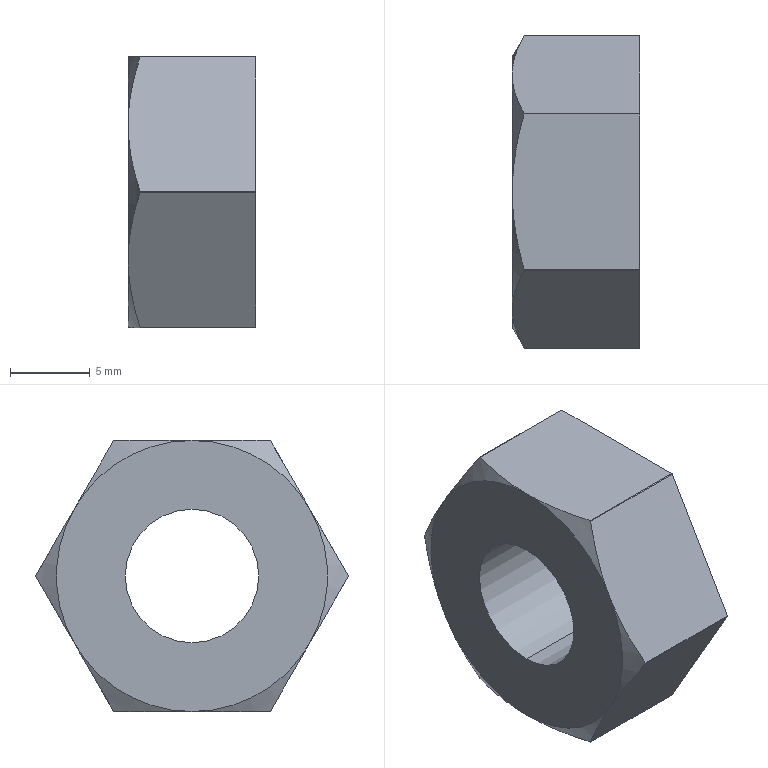Part | SolidWorks | features BaseBody 1 | 1 solid | 24 faces | box 8 x 19.6 x 17 mm | volume 1547 mm3 | cone 8 | cylinder 8 | plane 8 | commonest cylinder face diameters 19.6 x6 8.376 x2
STEP:
#1=CARTESIAN_POINT('',(-0.812,0.,-4.188));
#2=VERTEX_POINT('',#1);
#3=CARTESIAN_POINT('',(-0.812,0.,4.188));
#4=VERTEX_POINT('',#3);
#5=CARTESIAN_POINT('',(-0.812,0.,0.));
#6=DIRECTION('',(-1.,0.,0.));
#7=DIRECTION('',(0.,0.,1.));
#8=AXIS2_PLACEMENT_3D('',#5,#6,#7);
#9=CIRCLE('',#8,4.188);
#10=EDGE_CURVE('',#2,#4,#9,.T.);
#11=ORIENTED_EDGE('',*,*,#10,.T.);
#12=CARTESIAN_POINT('',(0.,0.,5.));
#13=VERTEX_POINT('',#12);
#14=CARTESIAN_POINT('',(0.,0.,5.));
#15=DIRECTION('',(0.7071,0.,0.7071));
#16=VECTOR('',#15,1000.);
#17=LINE('',#14,#16);
#18=EDGE_CURVE('',#4,#13,#17,.T.);
#19=ORIENTED_EDGE('',*,*,#18,.T.);
#20=CARTESIAN_POINT('',(0.,0.,-5.));
#21=VERTEX_POINT('',#20);
#22=CARTESIAN_POINT('',(0.,0.,0.));
#23=DIRECTION('',(-1.,0.,0.));
#24=DIRECTION('',(0.,0.,1.));
#25=AXIS2_PLACEMENT_3D('',#22,#23,#24);
#26=CIRCLE('',#25,5.);
#27=EDGE_CURVE('',#21,#13,#26,.T.);
#28=ORIENTED_EDGE('',*,*,#27,.F.);
#29=CARTESIAN_POINT('',(0.,0.,-5.));
#30=DIRECTION('',(0.7071,0.,-0.7071));
#31=VECTOR('',#30,1000.);
#32=LINE('',#29,#31);
#33=EDGE_CURVE('',#2,#21,#32,.T.);
#34=ORIENTED_EDGE('',*,*,#33,.F.);
#35=EDGE_LOOP('',(#11,#19,#28,#34));
#36=FACE_OUTER_BOUND('',#35,.T.);
#37=CARTESIAN_POINT('',(0.,0.,0.));
#38=DIRECTION('',(1.,0.,0.));
#39=DIRECTION('',(0.,0.,-1.));
#40=AXIS2_PLACEMENT_3D('',#37,#38,#39);
#41=CONICAL_SURFACE('',#40,5.,0.7854);
#42=ADVANCED_FACE('',(#36),#41,.F.);
#43=ORIENTED_EDGE('',*,*,#10,.F.);
#44=CARTESIAN_POINT('',(-8.,0.,-4.188));
#45=VERTEX_POINT('',#44);
#46=CARTESIAN_POINT('',(0.,0.,-4.188));
#47=DIRECTION('',(-1.,0.,0.));
#48=VECTOR('',#47,1000.);
#49=LINE('',#46,#48);
#50=EDGE_CURVE('',#2,#45,#49,.T.);
#51=ORIENTED_EDGE('',*,*,#50,.T.);
#52=CARTESIAN_POINT('',(-8.,0.,4.188));
#53=VERTEX_POINT('',#52);
#54=CARTESIAN_POINT('',(-8.,0.,0.));
#55=DIRECTION('',(-1.,0.,0.));
#56=DIRECTION('',(0.,0.,1.));
#57=AXIS2_PLACEMENT_3D('',#54,#55,#56);
#58=CIRCLE('',#57,4.188);
#59=EDGE_CURVE('',#45,#53,#58,.T.);
#60=ORIENTED_EDGE('',*,*,#59,.T.);
#61=CARTESIAN_POINT('',(0.,0.,4.188));
#62=DIRECTION('',(-1.,0.,0.));
#63=VECTOR('',#62,1000.);
#64=LINE('',#61,#63);
#65=EDGE_CURVE('',#4,#53,#64,.T.);
#66=ORIENTED_EDGE('',*,*,#65,.F.);
#67=EDGE_LOOP('',(#43,#51,#60,#66));
#68=FACE_OUTER_BOUND('',#67,.T.);
#69=CARTESIAN_POINT('',(0.,0.,0.));
#70=DIRECTION('',(-1.,0.,0.));
#71=DIRECTION('',(0.,0.,1.));
#72=AXIS2_PLACEMENT_3D('',#69,#70,#71);
#73=CYLINDRICAL_SURFACE('',#72,4.188);
#74=ADVANCED_FACE('',(#68),#73,.F.);
#75=ORIENTED_EDGE('',*,*,#27,.T.);
#76=CARTESIAN_POINT('',(0.,0.,0.));
#77=DIRECTION('',(-1.,0.,0.));
#78=DIRECTION('',(0.,0.,1.));
#79=AXIS2_PLACEMENT_3D('',#76,#77,#78);
#80=CIRCLE('',#79,5.);
#81=EDGE_CURVE('',#13,#21,#80,.T.);
#82=ORIENTED_EDGE('',*,*,#81,.T.);
#83=EDGE_LOOP('',(#75,#82));
#84=FACE_BOUND('',#83,.T.);
#85=CARTESIAN_POINT('',(0.,9.8,0.02596));
#86=VERTEX_POINT('',#85);
#87=CARTESIAN_POINT('',(0.,4.922,8.474));
#88=VERTEX_POINT('',#87);
#89=CARTESIAN_POINT('',(0.,9.815,0.));
#90=DIRECTION('',(0.,-0.5,0.866));
#91=VECTOR('',#90,1000.);
#92=LINE('',#89,#91);
#93=EDGE_CURVE('',#86,#88,#92,.T.);
#94=ORIENTED_EDGE('',*,*,#93,.T.);
#95=CARTESIAN_POINT('',(0.,4.877,8.5));
#96=VERTEX_POINT('',#95);
#97=CARTESIAN_POINT('',(0.,0.,0.));
#98=DIRECTION('',(-1.,0.,0.));
#99=DIRECTION('',(0.,0.,1.));
#100=AXIS2_PLACEMENT_3D('',#97,#98,#99);
#101=CIRCLE('',#100,9.8);
#102=EDGE_CURVE('',#96,#88,#101,.T.);
#103=ORIENTED_EDGE('',*,*,#102,.F.);
#104=CARTESIAN_POINT('',(0.,-4.877,8.5));
#105=VERTEX_POINT('',#104);
#106=CARTESIAN_POINT('',(0.,4.907,8.5));
#107=DIRECTION('',(0.,-1.,0.));
#108=VECTOR('',#107,1000.);
#109=LINE('',#106,#108);
#110=EDGE_CURVE('',#96,#105,#109,.T.);
#111=ORIENTED_EDGE('',*,*,#110,.T.);
#112=CARTESIAN_POINT('',(0.,-4.922,8.474));
#113=VERTEX_POINT('',#112);
#114=CARTESIAN_POINT('',(0.,0.,0.));
#115=DIRECTION('',(-1.,0.,0.));
#116=DIRECTION('',(0.,0.,1.));
#117=AXIS2_PLACEMENT_3D('',#114,#115,#116);
#118=CIRCLE('',#117,9.8);
#119=EDGE_CURVE('',#113,#105,#118,.T.);
#120=ORIENTED_EDGE('',*,*,#119,.F.);
#121=CARTESIAN_POINT('',(0.,-9.8,0.02596));
#122=VERTEX_POINT('',#121);
#123=CARTESIAN_POINT('',(0.,-4.907,8.5));
#124=DIRECTION('',(0.,-0.5,-0.866));
#125=VECTOR('',#124,1000.);
#126=LINE('',#123,#125);
#127=EDGE_CURVE('',#113,#122,#126,.T.);
#128=ORIENTED_EDGE('',*,*,#127,.T.);
#129=CARTESIAN_POINT('',(0.,-9.8,-0.02596));
#130=VERTEX_POINT('',#129);
#131=CARTESIAN_POINT('',(0.,0.,0.));
#132=DIRECTION('',(-1.,0.,0.));
#133=DIRECTION('',(0.,0.,1.));
#134=AXIS2_PLACEMENT_3D('',#131,#132,#133);
#135=CIRCLE('',#134,9.8);
#136=EDGE_CURVE('',#130,#122,#135,.T.);
#137=ORIENTED_EDGE('',*,*,#136,.F.);
#138=CARTESIAN_POINT('',(0.,-4.922,-8.474));
#139=VERTEX_POINT('',#138);
#140=CARTESIAN_POINT('',(0.,-9.815,0.));
#141=DIRECTION('',(0.,0.5,-0.866));
#142=VECTOR('',#141,1000.);
#143=LINE('',#140,#142);
#144=EDGE_CURVE('',#130,#139,#143,.T.);
#145=ORIENTED_EDGE('',*,*,#144,.T.);
#146=CARTESIAN_POINT('',(0.,-4.877,-8.5));
#147=VERTEX_POINT('',#146);
#148=CARTESIAN_POINT('',(0.,0.,0.));
#149=DIRECTION('',(-1.,0.,0.));
#150=DIRECTION('',(0.,0.,1.));
#151=AXIS2_PLACEMENT_3D('',#148,#149,#150);
#152=CIRCLE('',#151,9.8);
#153=EDGE_CURVE('',#147,#139,#152,.T.);
#154=ORIENTED_EDGE('',*,*,#153,.F.);
#155=CARTESIAN_POINT('',(0.,4.877,-8.5));
#156=VERTEX_POINT('',#155);
#157=CARTESIAN_POINT('',(0.,-4.907,-8.5));
#158=DIRECTION('',(0.,1.,0.));
#159=VECTOR('',#158,1000.);
#160=LINE('',#157,#159);
#161=EDGE_CURVE('',#147,#156,#160,.T.);
#162=ORIENTED_EDGE('',*,*,#161,.T.);
#163=CARTESIAN_POINT('',(0.,4.922,-8.474));
#164=VERTEX_POINT('',#163);
#165=CARTESIAN_POINT('',(0.,0.,0.));
#166=DIRECTION('',(-1.,0.,0.));
#167=DIRECTION('',(0.,0.,1.));
#168=AXIS2_PLACEMENT_3D('',#165,#166,#167);
#169=CIRCLE('',#168,9.8);
#170=EDGE_CURVE('',#164,#156,#169,.T.);
#171=ORIENTED_EDGE('',*,*,#170,.F.);
#172=CARTESIAN_POINT('',(0.,9.8,-0.02596));
#173=VERTEX_POINT('',#172);
#174=CARTESIAN_POINT('',(0.,4.907,-8.5));
#175=DIRECTION('',(0.,0.5,0.866));
#176=VECTOR('',#175,1000.);
#177=LINE('',#174,#176);
#178=EDGE_CURVE('',#164,#173,#177,.T.);
#179=ORIENTED_EDGE('',*,*,#178,.T.);
#180=CARTESIAN_POINT('',(0.,0.,0.));
#181=DIRECTION('',(-1.,0.,0.));
#182=DIRECTION('',(0.,0.,1.));
#183=AXIS2_PLACEMENT_3D('',#180,#181,#182);
#184=CIRCLE('',#183,9.8);
#185=EDGE_CURVE('',#86,#173,#184,.T.);
#186=ORIENTED_EDGE('',*,*,#185,.F.);
#187=EDGE_LOOP('',(#94,#103,#111,#120,#128,#137,#145,#154,#162,#171,#179,#186));
#188=FACE_OUTER_BOUND('',#187,.T.);
#189=CARTESIAN_POINT('',(0.,9.8,0.));
#190=DIRECTION('',(-1.,0.,0.));
#191=DIRECTION('',(0.,0.,1.));
#192=AXIS2_PLACEMENT_3D('',#189,#190,#191);
#193=PLANE('',#192);
#194=ADVANCED_FACE('',(#84,#188),#193,.F.);
#195=CARTESIAN_POINT('',(-7.249,9.8,0.02596));
#196=VERTEX_POINT('',#195);
#197=CARTESIAN_POINT('',(-8.,7.361,4.25));
#198=VERTEX_POINT('',#197);
#199=CARTESIAN_POINT('',(-7.249,9.8,0.02596));
#200=CARTESIAN_POINT('',(-7.479,9.401,0.7171));
#201=CARTESIAN_POINT('',(-7.668,8.999,1.413));
#202=CARTESIAN_POINT('',(-7.929,8.187,2.82));
#203=CARTESIAN_POINT('',(-8.,7.777,3.531));
#204=CARTESIAN_POINT('',(-8.,7.361,4.25));
#205=B_SPLINE_CURVE_WITH_KNOTS('',3,(#199,#200,#201,#202,#203,#204),.UNSPECIFIED.,.F.,.F.,(4,2,4),(0.000000483,0.002468,0.004935),.UNSPECIFIED.);
#206=EDGE_CURVE('',#196,#198,#205,.T.);
#207=ORIENTED_EDGE('',*,*,#206,.F.);
#208=CARTESIAN_POINT('',(-7.249,9.8,-0.02596));
#209=VERTEX_POINT('',#208);
#210=CARTESIAN_POINT('',(-7.249,0.,0.));
#211=DIRECTION('',(-1.,0.,0.));
#212=DIRECTION('',(0.,0.,1.));
#213=AXIS2_PLACEMENT_3D('',#210,#211,#212);
#214=CIRCLE('',#213,9.8);
#215=EDGE_CURVE('',#196,#209,#214,.T.);
#216=ORIENTED_EDGE('',*,*,#215,.T.);
#217=CARTESIAN_POINT('',(-8.,7.361,-4.25));
#218=VERTEX_POINT('',#217);
#219=CARTESIAN_POINT('',(-8.,7.361,-4.25));
#220=CARTESIAN_POINT('',(-8.,7.568,-3.892));
#221=CARTESIAN_POINT('',(-7.982,7.776,-3.532));
#222=CARTESIAN_POINT('',(-7.914,8.187,-2.819));
#223=CARTESIAN_POINT('',(-7.863,8.391,-2.466));
#224=CARTESIAN_POINT('',(-7.667,9.001,-1.41));
#225=CARTESIAN_POINT('',(-7.478,9.402,-0.7153));
#226=CARTESIAN_POINT('',(-7.249,9.8,-0.02596));
#227=B_SPLINE_CURVE_WITH_KNOTS('',3,(#219,#220,#221,#222,#223,#224,#225,#226),.UNSPECIFIED.,.F.,.F.,(4,2,2,4),(0.004935,0.006164,0.007393,0.00985),.UNSPECIFIED.);
#228=EDGE_CURVE('',#218,#209,#227,.T.);
#229=ORIENTED_EDGE('',*,*,#228,.F.);
#230=CARTESIAN_POINT('',(-8.,0.,0.));
#231=DIRECTION('',(-1.,0.,0.));
#232=DIRECTION('',(0.,0.,1.));
#233=AXIS2_PLACEMENT_3D('',#230,#231,#232);
#234=CIRCLE('',#233,8.5);
#235=EDGE_CURVE('',#198,#218,#234,.T.);
#236=ORIENTED_EDGE('',*,*,#235,.F.);
#237=EDGE_LOOP('',(#207,#216,#229,#236));
#238=FACE_OUTER_BOUND('',#237,.T.);
#239=CARTESIAN_POINT('',(-7.249,0.,0.));
#240=DIRECTION('',(1.,0.,0.));
#241=DIRECTION('',(0.,0.,-1.));
#242=AXIS2_PLACEMENT_3D('',#239,#240,#241);
#243=CONICAL_SURFACE('',#242,9.8,1.047);
#244=ADVANCED_FACE('',(#238),#243,.T.);
#245=CARTESIAN_POINT('',(-7.249,4.922,8.474));
#246=VERTEX_POINT('',#245);
#247=CARTESIAN_POINT('',(-8.,7.361,4.25));
#248=CARTESIAN_POINT('',(-8.,7.154,4.608));
#249=CARTESIAN_POINT('',(-7.982,6.946,4.968));
#250=CARTESIAN_POINT('',(-7.914,6.535,5.681));
#251=CARTESIAN_POINT('',(-7.863,6.331,6.034));
#252=CARTESIAN_POINT('',(-7.667,5.722,7.09));
#253=CARTESIAN_POINT('',(-7.478,5.32,7.785));
#254=CARTESIAN_POINT('',(-7.249,4.922,8.474));
#255=B_SPLINE_CURVE_WITH_KNOTS('',3,(#247,#248,#249,#250,#251,#252,#253,#254),.UNSPECIFIED.,.F.,.F.,(4,2,2,4),(0.004935,0.006164,0.007393,0.00985),.UNSPECIFIED.);
#256=EDGE_CURVE('',#198,#246,#255,.T.);
#257=ORIENTED_EDGE('',*,*,#256,.F.);
#258=CARTESIAN_POINT('',(-8.,0.,8.5));
#259=VERTEX_POINT('',#258);
#260=CARTESIAN_POINT('',(-8.,0.,0.));
#261=DIRECTION('',(-1.,0.,0.));
#262=DIRECTION('',(0.,0.,1.));
#263=AXIS2_PLACEMENT_3D('',#260,#261,#262);
#264=CIRCLE('',#263,8.5);
#265=EDGE_CURVE('',#259,#198,#264,.T.);
#266=ORIENTED_EDGE('',*,*,#265,.F.);
#267=CARTESIAN_POINT('',(-7.249,4.877,8.5));
#268=VERTEX_POINT('',#267);
#269=CARTESIAN_POINT('',(-7.249,4.877,8.5));
#270=CARTESIAN_POINT('',(-7.476,4.089,8.5));
#271=CARTESIAN_POINT('',(-7.665,3.29,8.5));
#272=CARTESIAN_POINT('',(-7.928,1.66,8.5));
#273=CARTESIAN_POINT('',(-8.,0.8245,8.5));
#274=CARTESIAN_POINT('',(-8.,0.,8.5));
#275=B_SPLINE_CURVE_WITH_KNOTS('',3,(#269,#270,#271,#272,#273,#274),.UNSPECIFIED.,.F.,.F.,(4,2,4),(0.00363,0.006092,0.008554),.UNSPECIFIED.);
#276=EDGE_CURVE('',#268,#259,#275,.T.);
#277=ORIENTED_EDGE('',*,*,#276,.F.);
#278=CARTESIAN_POINT('',(-7.249,0.,0.));
#279=DIRECTION('',(-1.,0.,0.));
#280=DIRECTION('',(0.,0.,1.));
#281=AXIS2_PLACEMENT_3D('',#278,#279,#280);
#282=CIRCLE('',#281,9.8);
#283=EDGE_CURVE('',#268,#246,#282,.T.);
#284=ORIENTED_EDGE('',*,*,#283,.T.);
#285=EDGE_LOOP('',(#257,#266,#277,#284));
#286=FACE_OUTER_BOUND('',#285,.T.);
#287=CARTESIAN_POINT('',(-7.249,0.,0.));
#288=DIRECTION('',(1.,0.,0.));
#289=DIRECTION('',(0.,0.,-1.));
#290=AXIS2_PLACEMENT_3D('',#287,#288,#289);
#291=CONICAL_SURFACE('',#290,9.8,1.047);
#292=ADVANCED_FACE('',(#286),#291,.T.);
#293=CARTESIAN_POINT('',(-7.249,4.922,-8.474));
#294=VERTEX_POINT('',#293);
#295=CARTESIAN_POINT('',(-7.249,4.922,-8.474));
#296=CARTESIAN_POINT('',(-7.479,5.322,-7.783));
#297=CARTESIAN_POINT('',(-7.668,5.723,-7.087));
#298=CARTESIAN_POINT('',(-7.929,6.536,-5.68));
#299=CARTESIAN_POINT('',(-8.,6.946,-4.969));
#300=CARTESIAN_POINT('',(-8.,7.361,-4.25));
#301=B_SPLINE_CURVE_WITH_KNOTS('',3,(#295,#296,#297,#298,#299,#300),.UNSPECIFIED.,.F.,.F.,(4,2,4),(0.000000717,0.002468,0.004935),.UNSPECIFIED.);
#302=EDGE_CURVE('',#294,#218,#301,.T.);
#303=ORIENTED_EDGE('',*,*,#302,.F.);
#304=CARTESIAN_POINT('',(-7.249,4.877,-8.5));
#305=VERTEX_POINT('',#304);
#306=CARTESIAN_POINT('',(-7.249,0.,0.));
#307=DIRECTION('',(-1.,0.,0.));
#308=DIRECTION('',(0.,0.,1.));
#309=AXIS2_PLACEMENT_3D('',#306,#307,#308);
#310=CIRCLE('',#309,9.8);
#311=EDGE_CURVE('',#294,#305,#310,.T.);
#312=ORIENTED_EDGE('',*,*,#311,.T.);
#313=CARTESIAN_POINT('',(-8.,0.,-8.5));
#314=VERTEX_POINT('',#313);
#315=CARTESIAN_POINT('',(-8.,0.,-8.5));
#316=CARTESIAN_POINT('',(-8.,0.8245,-8.5));
#317=CARTESIAN_POINT('',(-7.928,1.66,-8.5));
#318=CARTESIAN_POINT('',(-7.665,3.29,-8.5));
#319=CARTESIAN_POINT('',(-7.476,4.089,-8.5));
#320=CARTESIAN_POINT('',(-7.249,4.877,-8.5));
#321=B_SPLINE_CURVE_WITH_KNOTS('',3,(#315,#316,#317,#318,#319,#320),.UNSPECIFIED.,.F.,.F.,(4,2,4),(0.01372,0.01619,0.01866),.UNSPECIFIED.);
#322=EDGE_CURVE('',#314,#305,#321,.T.);
#323=ORIENTED_EDGE('',*,*,#322,.F.);
#324=CARTESIAN_POINT('',(-8.,0.,0.));
#325=DIRECTION('',(-1.,0.,0.));
#326=DIRECTION('',(0.,0.,1.));
#327=AXIS2_PLACEMENT_3D('',#324,#325,#326);
#328=CIRCLE('',#327,8.5);
#329=EDGE_CURVE('',#218,#314,#328,.T.);
#330=ORIENTED_EDGE('',*,*,#329,.F.);
#331=EDGE_LOOP('',(#303,#312,#323,#330));
#332=FACE_OUTER_BOUND('',#331,.T.);
#333=CARTESIAN_POINT('',(-7.249,0.,0.));
#334=DIRECTION('',(1.,0.,0.));
#335=DIRECTION('',(0.,0.,-1.));
#336=AXIS2_PLACEMENT_3D('',#333,#334,#335);
#337=CONICAL_SURFACE('',#336,9.8,1.047);
#338=ADVANCED_FACE('',(#332),#337,.T.);
#339=CARTESIAN_POINT('',(-7.249,-4.877,-8.5));
#340=VERTEX_POINT('',#339);
#341=CARTESIAN_POINT('',(-7.249,-4.877,-8.5));
#342=CARTESIAN_POINT('',(-7.477,-4.084,-8.5));
#343=CARTESIAN_POINT('',(-7.669,-3.271,-8.5));
#344=CARTESIAN_POINT('',(-7.93,-1.643,-8.5));
#345=CARTESIAN_POINT('',(-8.,-0.8241,-8.5));
#346=CARTESIAN_POINT('',(-8.,0.,-8.5));
#347=B_SPLINE_CURVE_WITH_KNOTS('',3,(#341,#342,#343,#344,#345,#346),.UNSPECIFIED.,.F.,.F.,(4,2,4),(0.008785,0.01125,0.01372),.UNSPECIFIED.);
#348=EDGE_CURVE('',#340,#314,#347,.T.);
#349=ORIENTED_EDGE('',*,*,#348,.F.);
#350=CARTESIAN_POINT('',(-7.249,-4.922,-8.474));
#351=VERTEX_POINT('',#350);
#352=CARTESIAN_POINT('',(-7.249,0.,0.));
#353=DIRECTION('',(-1.,0.,0.));
#354=DIRECTION('',(0.,0.,1.));
#355=AXIS2_PLACEMENT_3D('',#352,#353,#354);
#356=CIRCLE('',#355,9.8);
#357=EDGE_CURVE('',#340,#351,#356,.T.);
#358=ORIENTED_EDGE('',*,*,#357,.T.);
#359=CARTESIAN_POINT('',(-8.,-7.361,-4.25));
#360=VERTEX_POINT('',#359);
#361=CARTESIAN_POINT('',(-8.,-7.361,-4.25));
#362=CARTESIAN_POINT('',(-8.,-7.154,-4.608));
#363=CARTESIAN_POINT('',(-7.982,-6.946,-4.968));
#364=CARTESIAN_POINT('',(-7.914,-6.535,-5.681));
#365=CARTESIAN_POINT('',(-7.863,-6.331,-6.034));
#366=CARTESIAN_POINT('',(-7.667,-5.722,-7.09));
#367=CARTESIAN_POINT('',(-7.478,-5.32,-7.785));
#368=CARTESIAN_POINT('',(-7.249,-4.922,-8.474));
#369=B_SPLINE_CURVE_WITH_KNOTS('',3,(#361,#362,#363,#364,#365,#366,#367,#368),.UNSPECIFIED.,.F.,.F.,(4,2,2,4),(0.004935,0.006164,0.007393,0.00985),.UNSPECIFIED.);
#370=EDGE_CURVE('',#360,#351,#369,.T.);
#371=ORIENTED_EDGE('',*,*,#370,.F.);
#372=CARTESIAN_POINT('',(-8.,0.,0.));
#373=DIRECTION('',(-1.,0.,0.));
#374=DIRECTION('',(0.,0.,1.));
#375=AXIS2_PLACEMENT_3D('',#372,#373,#374);
#376=CIRCLE('',#375,8.5);
#377=EDGE_CURVE('',#314,#360,#376,.T.);
#378=ORIENTED_EDGE('',*,*,#377,.F.);
#379=EDGE_LOOP('',(#349,#358,#371,#378));
#380=FACE_OUTER_BOUND('',#379,.T.);
#381=CARTESIAN_POINT('',(-7.249,0.,0.));
#382=DIRECTION('',(1.,0.,0.));
#383=DIRECTION('',(0.,0.,-1.));
#384=AXIS2_PLACEMENT_3D('',#381,#382,#383);
#385=CONICAL_SURFACE('',#384,9.8,1.047);
#386=ADVANCED_FACE('',(#380),#385,.T.);
#387=CARTESIAN_POINT('',(-7.249,-9.8,-0.02596));
#388=VERTEX_POINT('',#387);
#389=CARTESIAN_POINT('',(-7.249,-9.8,-0.02596));
#390=CARTESIAN_POINT('',(-7.479,-9.401,-0.7171));
#391=CARTESIAN_POINT('',(-7.668,-8.999,-1.413));
#392=CARTESIAN_POINT('',(-7.929,-8.187,-2.82));
#393=CARTESIAN_POINT('',(-8.,-7.777,-3.531));
#394=CARTESIAN_POINT('',(-8.,-7.361,-4.25));
#395=B_SPLINE_CURVE_WITH_KNOTS('',3,(#389,#390,#391,#392,#393,#394),.UNSPECIFIED.,.F.,.F.,(4,2,4),(0.000000483,0.002468,0.004935),.UNSPECIFIED.);
#396=EDGE_CURVE('',#388,#360,#395,.T.);
#397=ORIENTED_EDGE('',*,*,#396,.F.);
#398=CARTESIAN_POINT('',(-7.249,-9.8,0.02596));
#399=VERTEX_POINT('',#398);
#400=CARTESIAN_POINT('',(-7.249,0.,0.));
#401=DIRECTION('',(-1.,0.,0.));
#402=DIRECTION('',(0.,0.,1.));
#403=AXIS2_PLACEMENT_3D('',#400,#401,#402);
#404=CIRCLE('',#403,9.8);
#405=EDGE_CURVE('',#388,#399,#404,.T.);
#406=ORIENTED_EDGE('',*,*,#405,.T.);
#407=CARTESIAN_POINT('',(-8.,-7.361,4.25));
#408=VERTEX_POINT('',#407);
#409=CARTESIAN_POINT('',(-8.,-7.361,4.25));
#410=CARTESIAN_POINT('',(-8.,-7.568,3.892));
#411=CARTESIAN_POINT('',(-7.982,-7.776,3.532));
#412=CARTESIAN_POINT('',(-7.914,-8.187,2.819));
#413=CARTESIAN_POINT('',(-7.863,-8.391,2.466));
#414=CARTESIAN_POINT('',(-7.667,-9.001,1.41));
#415=CARTESIAN_POINT('',(-7.478,-9.402,0.7153));
#416=CARTESIAN_POINT('',(-7.249,-9.8,0.02596));
#417=B_SPLINE_CURVE_WITH_KNOTS('',3,(#409,#410,#411,#412,#413,#414,#415,#416),.UNSPECIFIED.,.F.,.F.,(4,2,2,4),(0.004935,0.006164,0.007393,0.00985),.UNSPECIFIED.);
#418=EDGE_CURVE('',#408,#399,#417,.T.);
#419=ORIENTED_EDGE('',*,*,#418,.F.);
#420=CARTESIAN_POINT('',(-8.,0.,0.));
#421=DIRECTION('',(-1.,0.,0.));
#422=DIRECTION('',(0.,0.,1.));
#423=AXIS2_PLACEMENT_3D('',#420,#421,#422);
#424=CIRCLE('',#423,8.5);
#425=EDGE_CURVE('',#360,#408,#424,.T.);
#426=ORIENTED_EDGE('',*,*,#425,.F.);
#427=EDGE_LOOP('',(#397,#406,#419,#426));
#428=FACE_OUTER_BOUND('',#427,.T.);
#429=CARTESIAN_POINT('',(-7.249,0.,0.));
#430=DIRECTION('',(1.,0.,0.));
#431=DIRECTION('',(0.,0.,-1.));
#432=AXIS2_PLACEMENT_3D('',#429,#430,#431);
#433=CONICAL_SURFACE('',#432,9.8,1.047);
#434=ADVANCED_FACE('',(#428),#433,.T.);
#435=CARTESIAN_POINT('',(-7.249,-4.922,8.474));
#436=VERTEX_POINT('',#435);
#437=CARTESIAN_POINT('',(-7.249,-4.922,8.474));
#438=CARTESIAN_POINT('',(-7.479,-5.322,7.783));
#439=CARTESIAN_POINT('',(-7.668,-5.723,7.087));
#440=CARTESIAN_POINT('',(-7.929,-6.536,5.68));
#441=CARTESIAN_POINT('',(-8.,-6.946,4.969));
#442=CARTESIAN_POINT('',(-8.,-7.361,4.25));
#443=B_SPLINE_CURVE_WITH_KNOTS('',3,(#437,#438,#439,#440,#441,#442),.UNSPECIFIED.,.F.,.F.,(4,2,4),(0.000000717,0.002468,0.004935),.UNSPECIFIED.);
#444=EDGE_CURVE('',#436,#408,#443,.T.);
#445=ORIENTED_EDGE('',*,*,#444,.F.);
#446=CARTESIAN_POINT('',(-7.249,-4.877,8.5));
#447=VERTEX_POINT('',#446);
#448=CARTESIAN_POINT('',(-7.249,0.,0.));
#449=DIRECTION('',(-1.,0.,0.));
#450=DIRECTION('',(0.,0.,1.));
#451=AXIS2_PLACEMENT_3D('',#448,#449,#450);
#452=CIRCLE('',#451,9.8);
#453=EDGE_CURVE('',#436,#447,#452,.T.);
#454=ORIENTED_EDGE('',*,*,#453,.T.);
#455=CARTESIAN_POINT('',(-8.,0.,8.5));
#456=CARTESIAN_POINT('',(-8.,-0.8241,8.5));
#457=CARTESIAN_POINT('',(-7.93,-1.643,8.5));
#458=CARTESIAN_POINT('',(-7.669,-3.271,8.5));
#459=CARTESIAN_POINT('',(-7.477,-4.084,8.5));
#460=CARTESIAN_POINT('',(-7.249,-4.877,8.5));
#461=B_SPLINE_CURVE_WITH_KNOTS('',3,(#455,#456,#457,#458,#459,#460),.UNSPECIFIED.,.F.,.F.,(4,2,4),(0.008554,0.01101,0.01347),.UNSPECIFIED.);
#462=EDGE_CURVE('',#259,#447,#461,.T.);
#463=ORIENTED_EDGE('',*,*,#462,.F.);
#464=CARTESIAN_POINT('',(-8.,0.,0.));
#465=DIRECTION('',(-1.,0.,0.));
#466=DIRECTION('',(0.,0.,1.));
#467=AXIS2_PLACEMENT_3D('',#464,#465,#466);
#468=CIRCLE('',#467,8.5);
#469=EDGE_CURVE('',#408,#259,#468,.T.);
#470=ORIENTED_EDGE('',*,*,#469,.F.);
#471=EDGE_LOOP('',(#445,#454,#463,#470));
#472=FACE_OUTER_BOUND('',#471,.T.);
#473=CARTESIAN_POINT('',(-7.249,0.,0.));
#474=DIRECTION('',(1.,0.,0.));
#475=DIRECTION('',(0.,0.,-1.));
#476=AXIS2_PLACEMENT_3D('',#473,#474,#475);
#477=CONICAL_SURFACE('',#476,9.8,1.047);
#478=ADVANCED_FACE('',(#472),#477,.T.);
#479=CARTESIAN_POINT('',(0.,9.8,0.02596));
#480=DIRECTION('',(-1.,0.,0.));
#481=VECTOR('',#480,1000.);
#482=LINE('',#479,#481);
#483=EDGE_CURVE('',#86,#196,#482,.T.);
#484=ORIENTED_EDGE('',*,*,#483,.F.);
#485=ORIENTED_EDGE('',*,*,#185,.T.);
#486=CARTESIAN_POINT('',(0.,9.8,-0.02596));
#487=DIRECTION('',(1.,0.,0.));
#488=VECTOR('',#487,1000.);
#489=LINE('',#486,#488);
#490=EDGE_CURVE('',#209,#173,#489,.T.);
#491=ORIENTED_EDGE('',*,*,#490,.F.);
#492=ORIENTED_EDGE('',*,*,#215,.F.);
#493=EDGE_LOOP('',(#484,#485,#491,#492));
#494=FACE_OUTER_BOUND('',#493,.T.);
#495=CARTESIAN_POINT('',(0.,0.,0.));
#496=DIRECTION('',(-1.,0.,0.));
#497=DIRECTION('',(0.,0.,1.));
#498=AXIS2_PLACEMENT_3D('',#495,#496,#497);
#499=CYLINDRICAL_SURFACE('',#498,9.8);
#500=ADVANCED_FACE('',(#494),#499,.T.);
#501=CARTESIAN_POINT('',(0.,4.922,8.474));
#502=DIRECTION('',(1.,0.,0.));
#503=VECTOR('',#502,1000.);
#504=LINE('',#501,#503);
#505=EDGE_CURVE('',#246,#88,#504,.T.);
#506=ORIENTED_EDGE('',*,*,#505,.F.);
#507=ORIENTED_EDGE('',*,*,#283,.F.);
#508=CARTESIAN_POINT('',(0.,4.877,8.5));
#509=DIRECTION('',(-1.,0.,0.));
#510=VECTOR('',#509,1000.);
#511=LINE('',#508,#510);
#512=EDGE_CURVE('',#96,#268,#511,.T.);
#513=ORIENTED_EDGE('',*,*,#512,.F.);
#514=ORIENTED_EDGE('',*,*,#102,.T.);
#515=EDGE_LOOP('',(#506,#507,#513,#514));
#516=FACE_OUTER_BOUND('',#515,.T.);
#517=CARTESIAN_POINT('',(0.,0.,0.));
#518=DIRECTION('',(-1.,0.,0.));
#519=DIRECTION('',(0.,0.,1.));
#520=AXIS2_PLACEMENT_3D('',#517,#518,#519);
#521=CYLINDRICAL_SURFACE('',#520,9.8);
#522=ADVANCED_FACE('',(#516),#521,.T.);
#523=CARTESIAN_POINT('',(0.,4.922,-8.474));
#524=DIRECTION('',(-1.,0.,0.));
#525=VECTOR('',#524,1000.);
#526=LINE('',#523,#525);
#527=EDGE_CURVE('',#164,#294,#526,.T.);
#528=ORIENTED_EDGE('',*,*,#527,.F.);
#529=ORIENTED_EDGE('',*,*,#170,.T.);
#530=CARTESIAN_POINT('',(0.,4.877,-8.5));
#531=DIRECTION('',(1.,0.,0.));
#532=VECTOR('',#531,1000.);
#533=LINE('',#530,#532);
#534=EDGE_CURVE('',#305,#156,#533,.T.);
#535=ORIENTED_EDGE('',*,*,#534,.F.);
#536=ORIENTED_EDGE('',*,*,#311,.F.);
#537=EDGE_LOOP('',(#528,#529,#535,#536));
#538=FACE_OUTER_BOUND('',#537,.T.);
#539=CARTESIAN_POINT('',(0.,0.,0.));
#540=DIRECTION('',(-1.,0.,0.));
#541=DIRECTION('',(0.,0.,1.));
#542=AXIS2_PLACEMENT_3D('',#539,#540,#541);
#543=CYLINDRICAL_SURFACE('',#542,9.8);
#544=ADVANCED_FACE('',(#538),#543,.T.);
#545=CARTESIAN_POINT('',(0.,-4.877,-8.5));
#546=DIRECTION('',(-1.,0.,0.));
#547=VECTOR('',#546,1000.);
#548=LINE('',#545,#547);
#549=EDGE_CURVE('',#147,#340,#548,.T.);
#550=ORIENTED_EDGE('',*,*,#549,.F.);
#551=ORIENTED_EDGE('',*,*,#153,.T.);
#552=CARTESIAN_POINT('',(0.,-4.922,-8.474));
#553=DIRECTION('',(1.,0.,0.));
#554=VECTOR('',#553,1000.);
#555=LINE('',#552,#554);
#556=EDGE_CURVE('',#351,#139,#555,.T.);
#557=ORIENTED_EDGE('',*,*,#556,.F.);
#558=ORIENTED_EDGE('',*,*,#357,.F.);
#559=EDGE_LOOP('',(#550,#551,#557,#558));
#560=FACE_OUTER_BOUND('',#559,.T.);
#561=CARTESIAN_POINT('',(0.,0.,0.));
#562=DIRECTION('',(-1.,0.,0.));
#563=DIRECTION('',(0.,0.,1.));
#564=AXIS2_PLACEMENT_3D('',#561,#562,#563);
#565=CYLINDRICAL_SURFACE('',#564,9.8);
#566=ADVANCED_FACE('',(#560),#565,.T.);
#567=CARTESIAN_POINT('',(0.,-9.8,-0.02596));
#568=DIRECTION('',(-1.,0.,0.));
#569=VECTOR('',#568,1000.);
#570=LINE('',#567,#569);
#571=EDGE_CURVE('',#130,#388,#570,.T.);
#572=ORIENTED_EDGE('',*,*,#571,.F.);
#573=ORIENTED_EDGE('',*,*,#136,.T.);
#574=CARTESIAN_POINT('',(0.,-9.8,0.02596));
#575=DIRECTION('',(1.,0.,0.));
#576=VECTOR('',#575,1000.);
#577=LINE('',#574,#576);
#578=EDGE_CURVE('',#399,#122,#577,.T.);
#579=ORIENTED_EDGE('',*,*,#578,.F.);
#580=ORIENTED_EDGE('',*,*,#405,.F.);
#581=EDGE_LOOP('',(#572,#573,#579,#580));
#582=FACE_OUTER_BOUND('',#581,.T.);
#583=CARTESIAN_POINT('',(0.,0.,0.));
#584=DIRECTION('',(-1.,0.,0.));
#585=DIRECTION('',(0.,0.,1.));
#586=AXIS2_PLACEMENT_3D('',#583,#584,#585);
#587=CYLINDRICAL_SURFACE('',#586,9.8);
#588=ADVANCED_FACE('',(#582),#587,.T.);
#589=CARTESIAN_POINT('',(0.,-4.922,8.474));
#590=DIRECTION('',(-1.,0.,0.));
#591=VECTOR('',#590,1000.);
#592=LINE('',#589,#591);
#593=EDGE_CURVE('',#113,#436,#592,.T.);
#594=ORIENTED_EDGE('',*,*,#593,.F.);
#595=ORIENTED_EDGE('',*,*,#119,.T.);
#596=CARTESIAN_POINT('',(0.,-4.877,8.5));
#597=DIRECTION('',(1.,0.,0.));
#598=VECTOR('',#597,1000.);
#599=LINE('',#596,#598);
#600=EDGE_CURVE('',#447,#105,#599,.T.);
#601=ORIENTED_EDGE('',*,*,#600,.F.);
#602=ORIENTED_EDGE('',*,*,#453,.F.);
#603=EDGE_LOOP('',(#594,#595,#601,#602));
#604=FACE_OUTER_BOUND('',#603,.T.);
#605=CARTESIAN_POINT('',(0.,0.,0.));
#606=DIRECTION('',(-1.,0.,0.));
#607=DIRECTION('',(0.,0.,1.));
#608=AXIS2_PLACEMENT_3D('',#605,#606,#607);
#609=CYLINDRICAL_SURFACE('',#608,9.8);
#610=ADVANCED_FACE('',(#604),#609,.T.);
#611=ORIENTED_EDGE('',*,*,#265,.T.);
#612=ORIENTED_EDGE('',*,*,#235,.T.);
#613=ORIENTED_EDGE('',*,*,#329,.T.);
#614=ORIENTED_EDGE('',*,*,#377,.T.);
#615=ORIENTED_EDGE('',*,*,#425,.T.);
#616=ORIENTED_EDGE('',*,*,#469,.T.);
#617=EDGE_LOOP('',(#611,#612,#613,#614,#615,#616));
#618=FACE_OUTER_BOUND('',#617,.T.);
#619=CARTESIAN_POINT('',(-8.,0.,0.));
#620=DIRECTION('',(-1.,0.,0.));
#621=DIRECTION('',(0.,0.,1.));
#622=AXIS2_PLACEMENT_3D('',#619,#620,#621);
#623=CIRCLE('',#622,4.188);
#624=EDGE_CURVE('',#53,#45,#623,.T.);
#625=ORIENTED_EDGE('',*,*,#624,.F.);
#626=ORIENTED_EDGE('',*,*,#59,.F.);
#627=EDGE_LOOP('',(#625,#626));
#628=FACE_BOUND('',#627,.T.);
#629=CARTESIAN_POINT('',(-8.,0.,0.));
#630=DIRECTION('',(1.,0.,0.));
#631=DIRECTION('',(0.,0.,-1.));
#632=AXIS2_PLACEMENT_3D('',#629,#630,#631);
#633=PLANE('',#632);
#634=ADVANCED_FACE('',(#618,#628),#633,.F.);
#635=ORIENTED_EDGE('',*,*,#50,.F.);
#636=CARTESIAN_POINT('',(-0.812,0.,0.));
#637=DIRECTION('',(-1.,0.,0.));
#638=DIRECTION('',(0.,0.,1.));
#639=AXIS2_PLACEMENT_3D('',#636,#637,#638);
#640=CIRCLE('',#639,4.188);
#641=EDGE_CURVE('',#4,#2,#640,.T.);
#642=ORIENTED_EDGE('',*,*,#641,.F.);
#643=ORIENTED_EDGE('',*,*,#65,.T.);
#644=ORIENTED_EDGE('',*,*,#624,.T.);
#645=EDGE_LOOP('',(#635,#642,#643,#644));
#646=FACE_OUTER_BOUND('',#645,.T.);
#647=CARTESIAN_POINT('',(0.,0.,0.));
#648=DIRECTION('',(-1.,0.,0.));
#649=DIRECTION('',(0.,0.,1.));
#650=AXIS2_PLACEMENT_3D('',#647,#648,#649);
#651=CYLINDRICAL_SURFACE('',#650,4.188);
#652=ADVANCED_FACE('',(#646),#651,.F.);
#653=ORIENTED_EDGE('',*,*,#18,.F.);
#654=ORIENTED_EDGE('',*,*,#641,.T.);
#655=ORIENTED_EDGE('',*,*,#33,.T.);
#656=ORIENTED_EDGE('',*,*,#81,.F.);
#657=EDGE_LOOP('',(#653,#654,#655,#656));
#658=FACE_OUTER_BOUND('',#657,.T.);
#659=CARTESIAN_POINT('',(0.,0.,0.));
#660=DIRECTION('',(1.,0.,0.));
#661=DIRECTION('',(0.,0.,-1.));
#662=AXIS2_PLACEMENT_3D('',#659,#660,#661);
#663=CONICAL_SURFACE('',#662,5.,0.7854);
#664=ADVANCED_FACE('',(#658),#663,.F.);
#665=ORIENTED_EDGE('',*,*,#512,.T.);
#666=ORIENTED_EDGE('',*,*,#276,.T.);
#667=ORIENTED_EDGE('',*,*,#462,.T.);
#668=ORIENTED_EDGE('',*,*,#600,.T.);
#669=ORIENTED_EDGE('',*,*,#110,.F.);
#670=EDGE_LOOP('',(#665,#666,#667,#668,#669));
#671=FACE_OUTER_BOUND('',#670,.T.);
#672=CARTESIAN_POINT('',(-8.,4.907,8.5));
#673=DIRECTION('',(0.,0.,1.));
#674=DIRECTION('',(1.,0.,0.));
#675=AXIS2_PLACEMENT_3D('',#672,#673,#674);
#676=PLANE('',#675);
#677=ADVANCED_FACE('',(#671),#676,.T.);
#678=ORIENTED_EDGE('',*,*,#593,.T.);
#679=ORIENTED_EDGE('',*,*,#444,.T.);
#680=ORIENTED_EDGE('',*,*,#418,.T.);
#681=ORIENTED_EDGE('',*,*,#578,.T.);
#682=ORIENTED_EDGE('',*,*,#127,.F.);
#683=EDGE_LOOP('',(#678,#679,#680,#681,#682));
#684=FACE_OUTER_BOUND('',#683,.T.);
#685=CARTESIAN_POINT('',(-8.,-4.907,8.5));
#686=DIRECTION('',(0.,-0.866,0.5));
#687=DIRECTION('',(0.,-0.5,-0.866));
#688=AXIS2_PLACEMENT_3D('',#685,#686,#687);
#689=PLANE('',#688);
#690=ADVANCED_FACE('',(#684),#689,.T.);
#691=ORIENTED_EDGE('',*,*,#571,.T.);
#692=ORIENTED_EDGE('',*,*,#396,.T.);
#693=ORIENTED_EDGE('',*,*,#370,.T.);
#694=ORIENTED_EDGE('',*,*,#556,.T.);
#695=ORIENTED_EDGE('',*,*,#144,.F.);
#696=EDGE_LOOP('',(#691,#692,#693,#694,#695));
#697=FACE_OUTER_BOUND('',#696,.T.);
#698=CARTESIAN_POINT('',(-8.,-9.815,0.));
#699=DIRECTION('',(0.,-0.866,-0.5));
#700=DIRECTION('',(0.,0.5,-0.866));
#701=AXIS2_PLACEMENT_3D('',#698,#699,#700);
#702=PLANE('',#701);
#703=ADVANCED_FACE('',(#697),#702,.T.);
#704=ORIENTED_EDGE('',*,*,#549,.T.);
#705=ORIENTED_EDGE('',*,*,#348,.T.);
#706=ORIENTED_EDGE('',*,*,#322,.T.);
#707=ORIENTED_EDGE('',*,*,#534,.T.);
#708=ORIENTED_EDGE('',*,*,#161,.F.);
#709=EDGE_LOOP('',(#704,#705,#706,#707,#708));
#710=FACE_OUTER_BOUND('',#709,.T.);
#711=CARTESIAN_POINT('',(-8.,-4.907,-8.5));
#712=DIRECTION('',(0.,0.,-1.));
#713=DIRECTION('',(-1.,0.,0.));
#714=AXIS2_PLACEMENT_3D('',#711,#712,#713);
#715=PLANE('',#714);
#716=ADVANCED_FACE('',(#710),#715,.T.);
#717=ORIENTED_EDGE('',*,*,#527,.T.);
#718=ORIENTED_EDGE('',*,*,#302,.T.);
#719=ORIENTED_EDGE('',*,*,#228,.T.);
#720=ORIENTED_EDGE('',*,*,#490,.T.);
#721=ORIENTED_EDGE('',*,*,#178,.F.);
#722=EDGE_LOOP('',(#717,#718,#719,#720,#721));
#723=FACE_OUTER_BOUND('',#722,.T.);
#724=CARTESIAN_POINT('',(-8.,4.907,-8.5));
#725=DIRECTION('',(0.,0.866,-0.5));
#726=DIRECTION('',(0.,0.5,0.866));
#727=AXIS2_PLACEMENT_3D('',#724,#725,#726);
#728=PLANE('',#727);
#729=ADVANCED_FACE('',(#723),#728,.T.);
#730=ORIENTED_EDGE('',*,*,#483,.T.);
#731=ORIENTED_EDGE('',*,*,#206,.T.);
#732=ORIENTED_EDGE('',*,*,#256,.T.);
#733=ORIENTED_EDGE('',*,*,#505,.T.);
#734=ORIENTED_EDGE('',*,*,#93,.F.);
#735=EDGE_LOOP('',(#730,#731,#732,#733,#734));
#736=FACE_OUTER_BOUND('',#735,.T.);
#737=CARTESIAN_POINT('',(-8.,9.815,0.));
#738=DIRECTION('',(0.,0.866,0.5));
#739=DIRECTION('',(0.,-0.5,0.866));
#740=AXIS2_PLACEMENT_3D('',#737,#738,#739);
#741=PLANE('',#740);
#742=ADVANCED_FACE('',(#736),#741,.T.);
#743=CLOSED_SHELL('',(#42,#74,#194,#244,#292,#338,#386,#434,#478,#500,#522,#544,#566,#588,#610,#634,#652,#664,#677,#690,#703,#716,#729,#742));
#744=MANIFOLD_SOLID_BREP('',#743);
#745=CARTESIAN_POINT('',(0.,0.,0.));
#746=DIRECTION('',(0.,0.,1.));
#747=DIRECTION('',(1.,0.,0.));
#748=AXIS2_PLACEMENT_3D('',#745,#746,#747);
#749=(LENGTH_UNIT()NAMED_UNIT(*)SI_UNIT(.MILLI.,.METRE.));
#750=UNCERTAINTY_MEASURE_WITH_UNIT(LENGTH_MEASURE(0.00001),#749,'','');
#751=(NAMED_UNIT(*)PLANE_ANGLE_UNIT()SI_UNIT($,.RADIAN.));
#752=(NAMED_UNIT(*)SI_UNIT($,.STERADIAN.)SOLID_ANGLE_UNIT());
#753=(GEOMETRIC_REPRESENTATION_CONTEXT(3)GLOBAL_UNCERTAINTY_ASSIGNED_CONTEXT((#750))GLOBAL_UNIT_ASSIGNED_CONTEXT((#749,#751,#752))REPRESENTATION_CONTEXT('',''));
#754=ADVANCED_BREP_SHAPE_REPRESENTATION('',(#744,#748),#753);